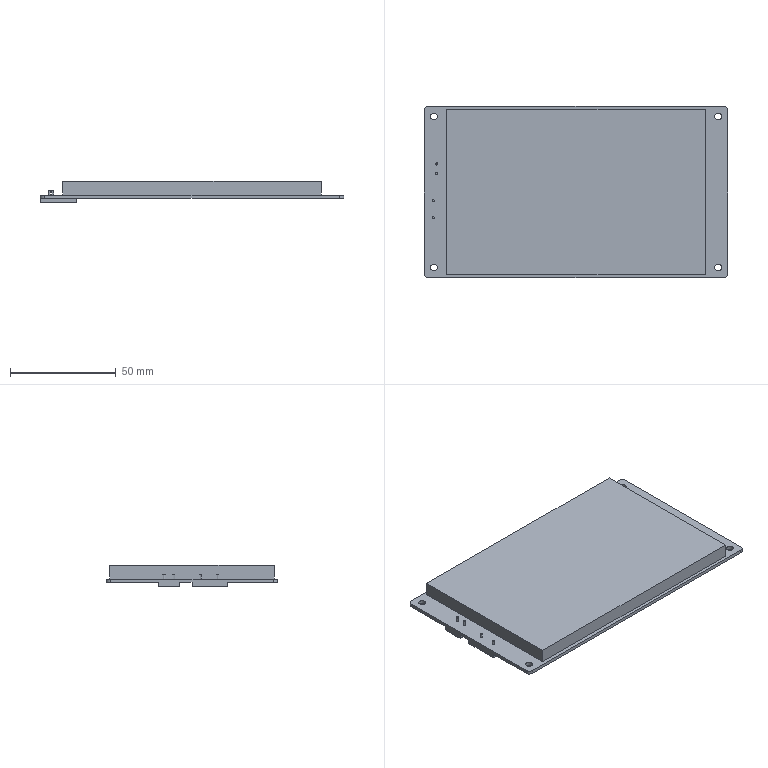Part | STEP file | Screen OCM800480T500 | 6 solids | 40 faces | box 143.47 x 81 x 10.1 mm | volume 81087 mm3 | plane 28 | cylinder 12 | commonest cylinder face diameters 1 x4 3.2 x4 4 x4